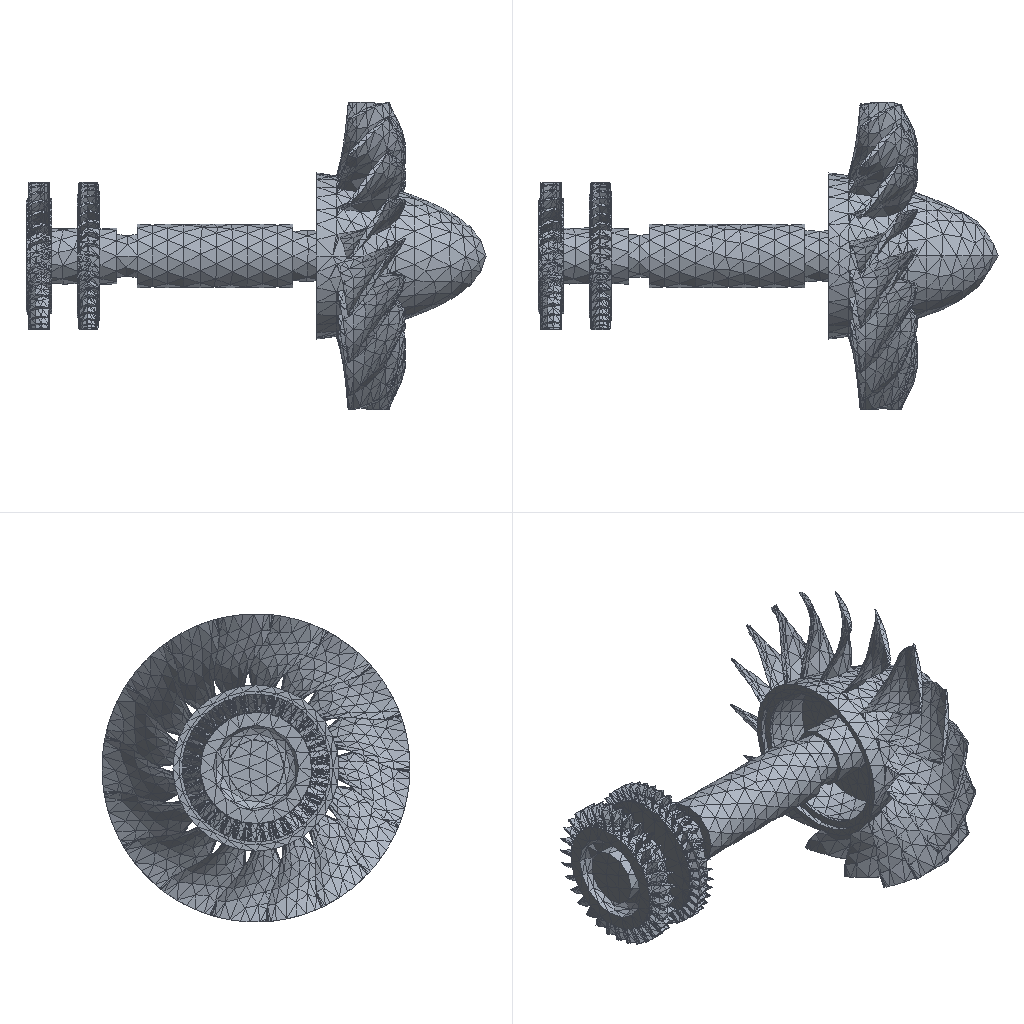Simulation study | ansys workbench
Set-up summary:
category,name,step,type,value,unit,region
solver,ansys_workbench
units,mm-N-s-tonne (MPa),,stated,"/units,MPA"
analysis,deck-1/LS1,,modal,method=lanb; n_modes=4
load_step,deck-1/LS1,deck-1/LS1,modal
analysis,deck-2/LS1,,modal,method=qrdamp; n_modes=4
load_step,deck-2/LS1,deck-2/LS1,modal
load_step,deck-2/LS1,deck-2/LS1,modal
load_step,deck-2/LS1,deck-2/LS1,modal
load_step,deck-2/LS1,deck-2/LS1,modal
mesh,deck-1.dat,,nodes,56734
mesh,deck-1.dat,,elements,28095
element_type,SOLID187,,,27427,,deck-1.dat
element_type,CONTA174,,,388,,deck-1.dat
element_type,TARGE170,,,280,,deck-1.dat
mesh,deck-2.dat,,nodes,56736
mesh,deck-2.dat,,elements,28095
element_type,SOLID187,,,27427,,deck-2.dat
element_type,CONTA174,,,388,,deck-2.dat
element_type,TARGE170,,,280,,deck-2.dat
material,Structural Steel,,E,200000,tonne s^-2 mm^-1
material,Structural Steel,,nu,0.3
material,Structural Steel,,density,7.85e-09,tonne mm^-3
material,Structural Steel,,conductivity,60.5,tonne mm s^-3 C^-1
material,Structural Steel,,specific_heat,4.34e+08,mm^2 s^-2 C^-1
material,Structural Steel,,cte,1.2e-05,C^-1
material,Structural Steel,,permeability,10000
material,Structural Steel,,resistivity,0.00017,ohm mm
bc,"Create Bearing Connection ""? ? Component2\710500""",deck-1/model,fixed,[dofs=ALL n=2],,node list
bc,Construct Remote Displacement,deck-1/model,fixed,[dofs=UX n=2],,node list
bc,"Create Bearing Connection ""? ? Component2\710500""",deck-2/model,fixed,[dofs=ALL n=2],,node list
bc,Construct Remote Displacement,deck-2/model,fixed,[dofs=UX n=2],,node list
contact,Contact Region,,bonded (always),element=CONTA174
contact,Contact Region 2,,bonded (always),element=CONTA174
contact,Contact Region 3,,bonded (always),element=CONTA174
contact,contact 4,,bonded (always),element=CONTA174
contact,contact 5,,bonded (always),element=CONTA174
contact,contact 6,,bonded (always),element=CONTA174
contact,contact 7,,bonded (always),element=CONTA174
contact,Contact Region,,bonded (always),element=CONTA174
contact,Contact Region 2,,bonded (always),element=CONTA174
contact,Contact Region 3,,bonded (always),element=CONTA174
contact,contact 4,,bonded (always),element=CONTA174
contact,contact 5,,bonded (always),element=CONTA174
contact,contact 6,,bonded (always),element=CONTA174
contact,contact 7,,bonded (always),element=CONTA174
named_set,REMOTEDISPALL,,node,2
named_set,REMOTEDISPALL,,node,2
Results summary:
result,analyses[0].index,,,1
result,analyses[0].system,,,SYS
result,analyses[0].deck,,,deck-1.dat
result,analyses[0].solve_status,,,completed
result,analyses[0].analysis_type,,,modal
result,analyses[0].physics,,,mechanical
result,analyses[0].unit_system,,,"NMM: mm, ton, N, s, mV, mA, degC"
result,analyses[0].n_sets,,,4
result,analyses[0].modal_frequencies_hz[1],,,12.29
result,analyses[0].modal_frequencies_hz[2],,,203.03
result,analyses[0].modal_frequencies_hz[3],,,203.076
result,analyses[0].modal_frequencies_hz[4],,,393.54
result,analyses[1].index,,,2
result,analyses[1].system,,,SYS-1
result,analyses[1].deck,,,deck-2.dat
result,analyses[1].solve_status,,,completed
result,analyses[1].analysis_type,,,modal
result,analyses[1].physics,,,mechanical
result,analyses[1].unit_system,,,"NMM: mm, ton, N, s, mV, mA, degC"
result,analyses[1].n_sets,,,16
result,analyses[1].modal_frequencies_hz[1],,,12.29
result,analyses[1].modal_frequencies_hz[2],,,202.917
result,analyses[1].modal_frequencies_hz[3],,,203.19
result,analyses[1].modal_frequencies_hz[4],,,393.54
result,analyses[1].modal_frequencies_hz[5],,,12.29
result,analyses[1].modal_frequencies_hz[6],,,201.711
result,analyses[1].modal_frequencies_hz[7],,,204.402
result,analyses[1].modal_frequencies_hz[8],,,393.544
result,analyses[1].modal_frequencies_hz[9],,,12.29
result,analyses[1].modal_frequencies_hz[10],,,189.964
result,analyses[1].modal_frequencies_hz[11],,,216.833
result,analyses[1].modal_frequencies_hz[12],,,393.923
result,analyses[1].modal_frequencies_hz[13],,,12.29
result,analyses[1].modal_frequencies_hz[14],,,177.647
result,analyses[1].modal_frequencies_hz[15],,,231.171
result,analyses[1].modal_frequencies_hz[16],,,395.109
result,geometry_export[0][0],,,.step
result,geometry_export[0][1],,,ok
result,geometry_export[0][2],,,4